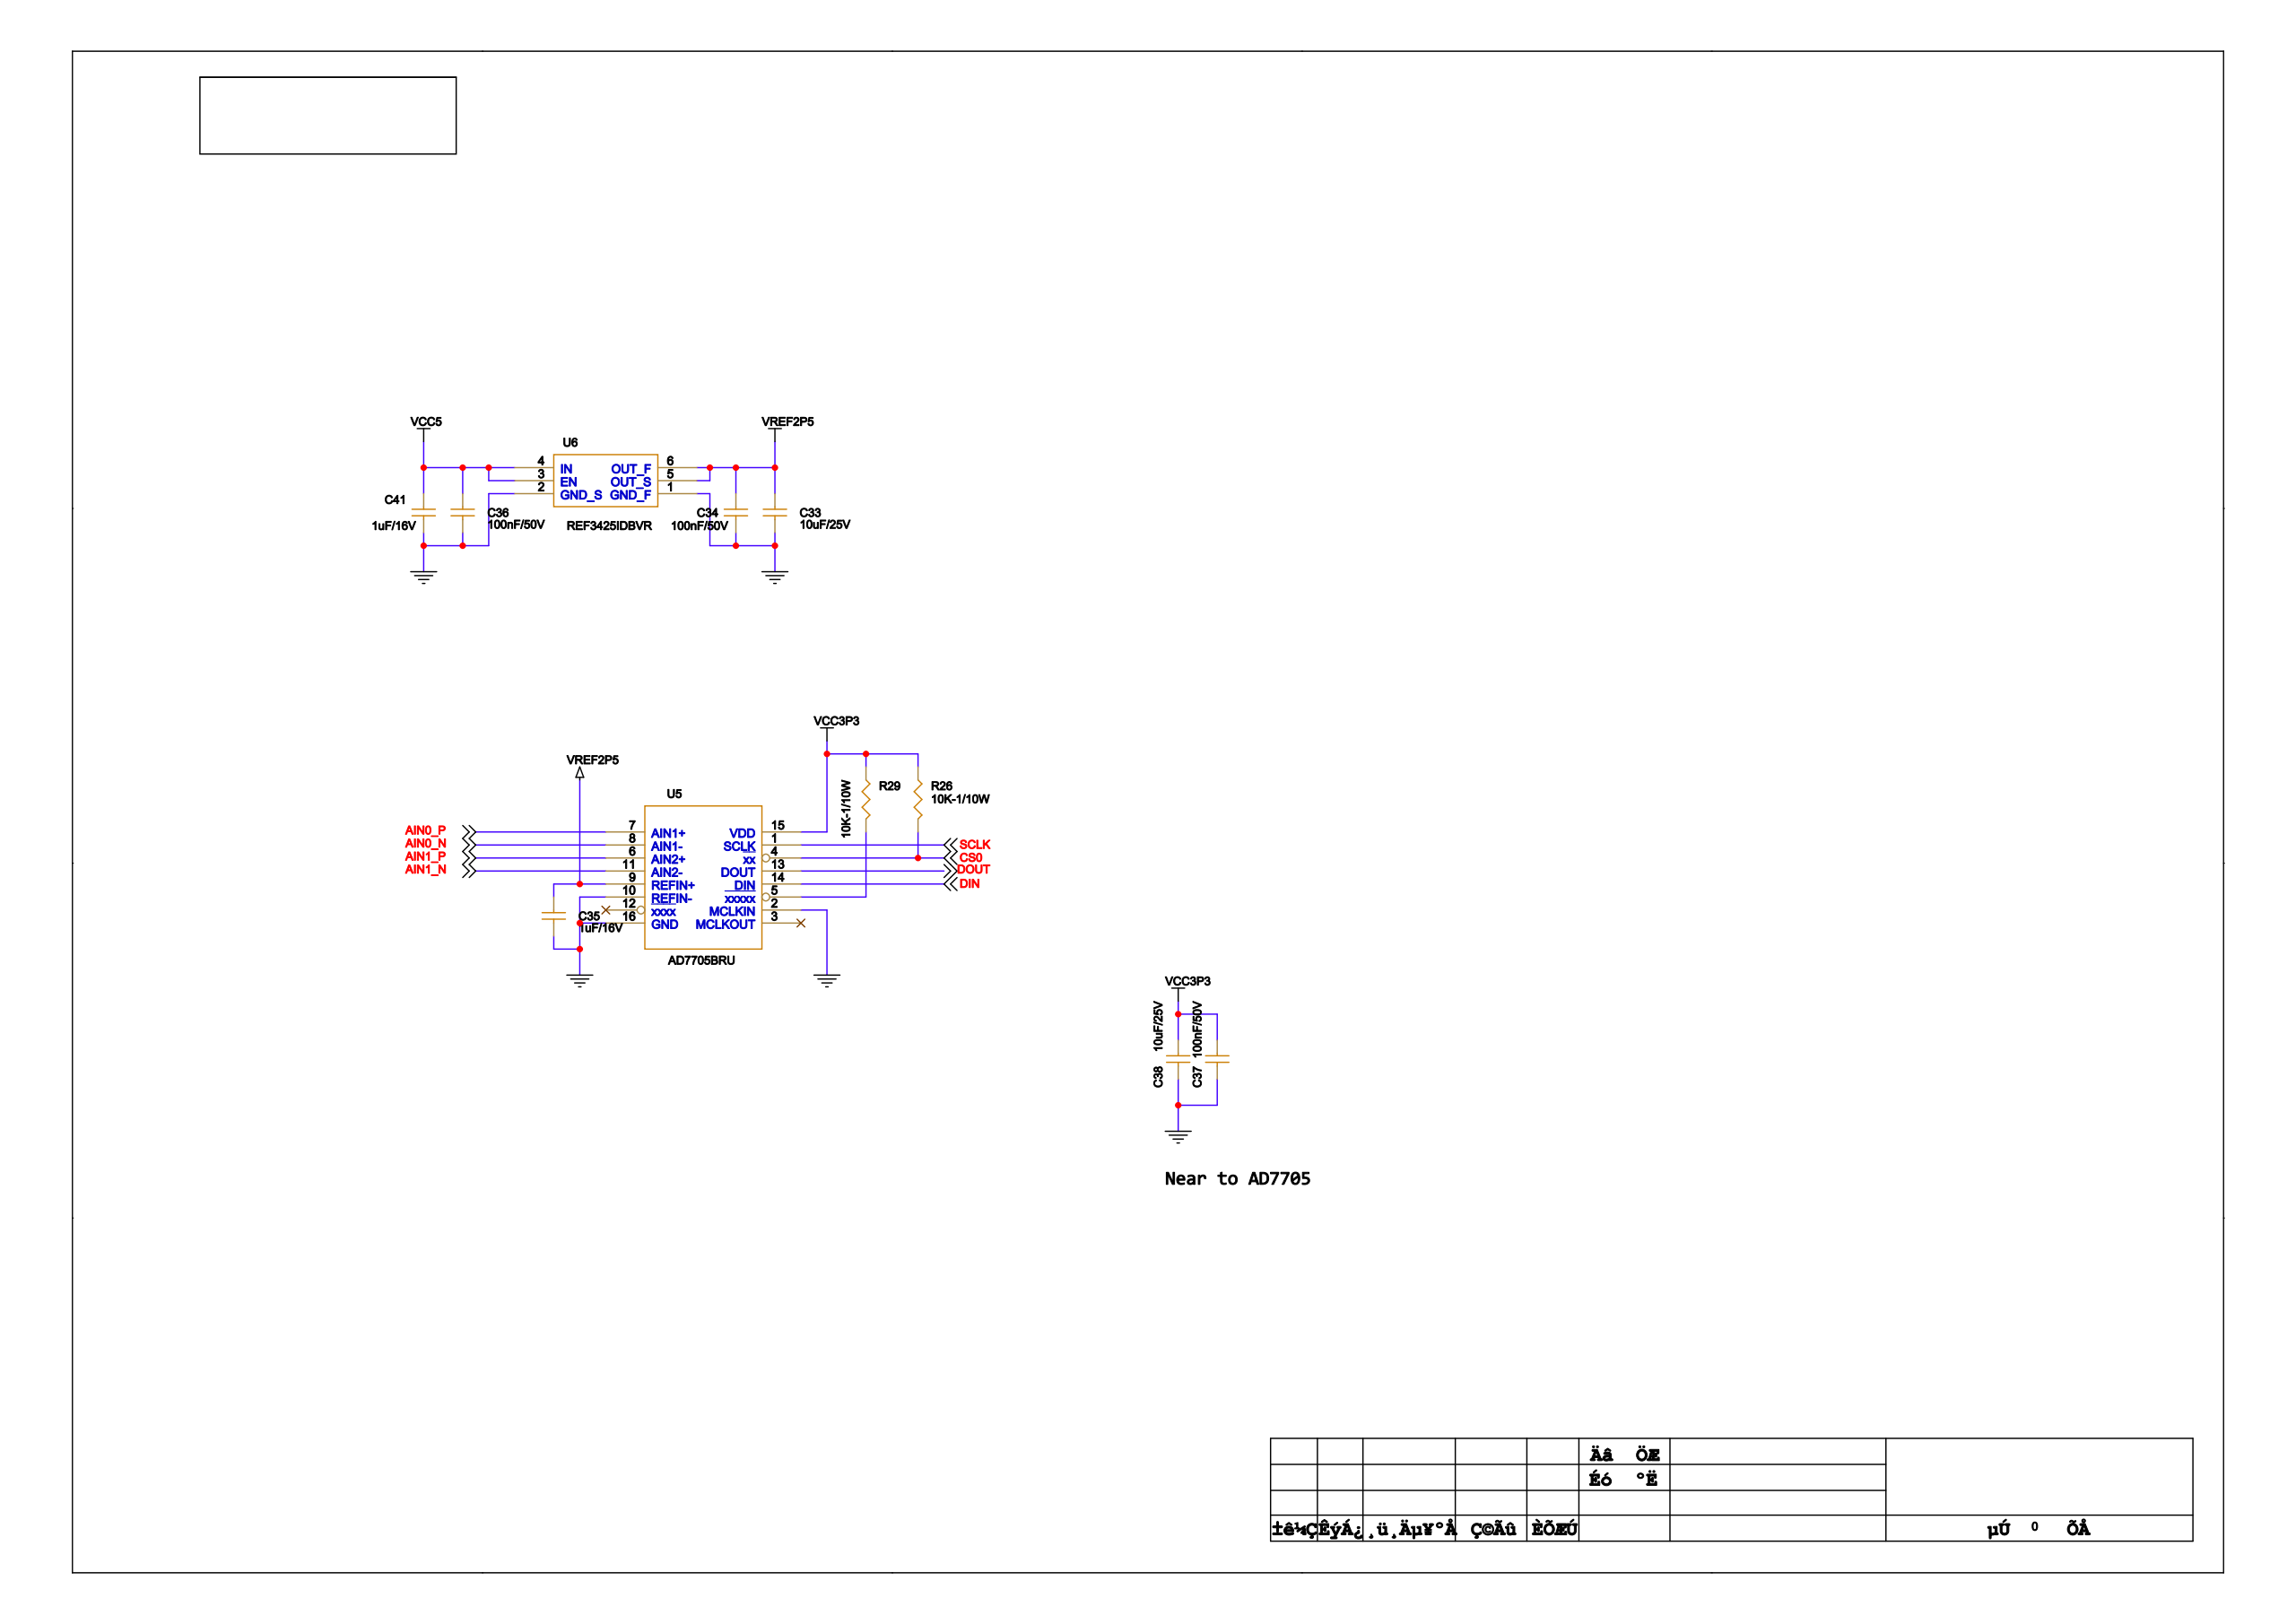Circuit board | Cadence Allegro | 65 parts | 41 nets | one sheet of the schematic
Parts on this sheet (reference | value | footprint):
C33 | 10uF/25V | C0805
C34 | 100nF/50V | C0603
C35 | 1uF/16V | C0603
C36 | 100nF/50V | C0603
C37 | 100nF/50V | C0603
C38 | 10uF/25V | C0805
C41 | 1uF/16V | C0603
R26 | 10K-1/10W | R0603
R29 | 10K-1/10W | R0603
U5 | AD7705BRU | TSSOP16_P0_65
U6 | REF3425IDBVR | SOT23_6
Nets of these parts (net: part-pin ...):
AIN0_P: U5-7
GND: C33-2 C34-2 C35-2 C36-2 C37-2 C38-2 C41-2 U5-2 U5-10 U5-16 U6-1 U6-2
AIN1_P: U5-6
AIN1_N: U5-11
AIN0_N: U5-8
VCC5: C36-1 C41-1 U6-3 U6-4
VCC3P3: C37-1 C38-1 R26-1 R29-1 U5-15
VREF2P5: C33-1 C34-1 C35-1 U5-9 U6-5 U6-6
CS0: R26-2 U5-4
SCLK: U5-1
DOUT: U5-13
DIN: U5-14
N7798739: R29-2 U5-5